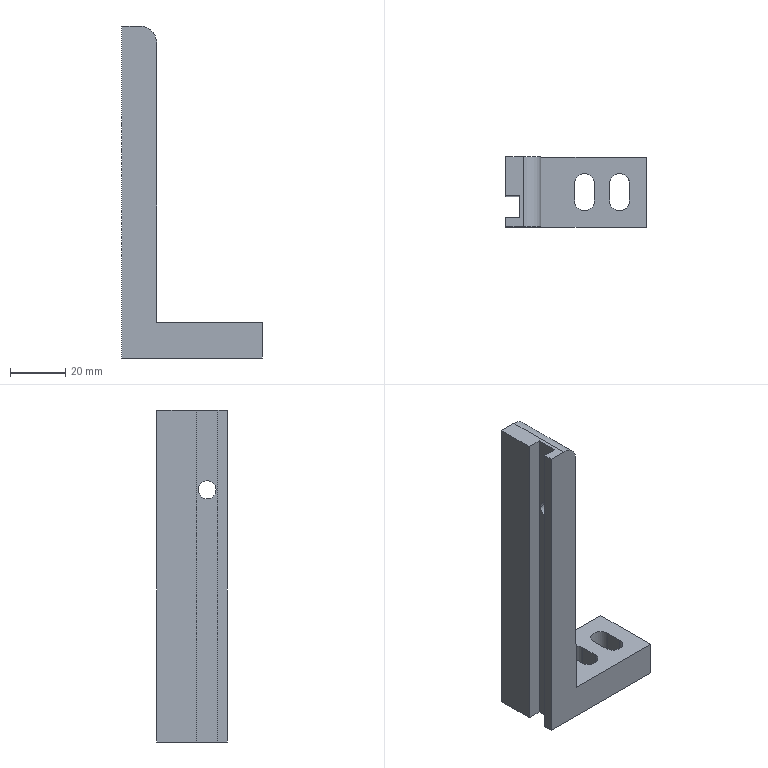Part | STEP file | 1_id1310_x_t | 1 solid | 27 faces | box 50.8 x 25.4 x 120.024 mm | volume 43266 mm3 | plane 18 | cylinder 9 | commonest cylinder face diameters 7.112 x4 6.5 x2 11 x2 12.693 x1